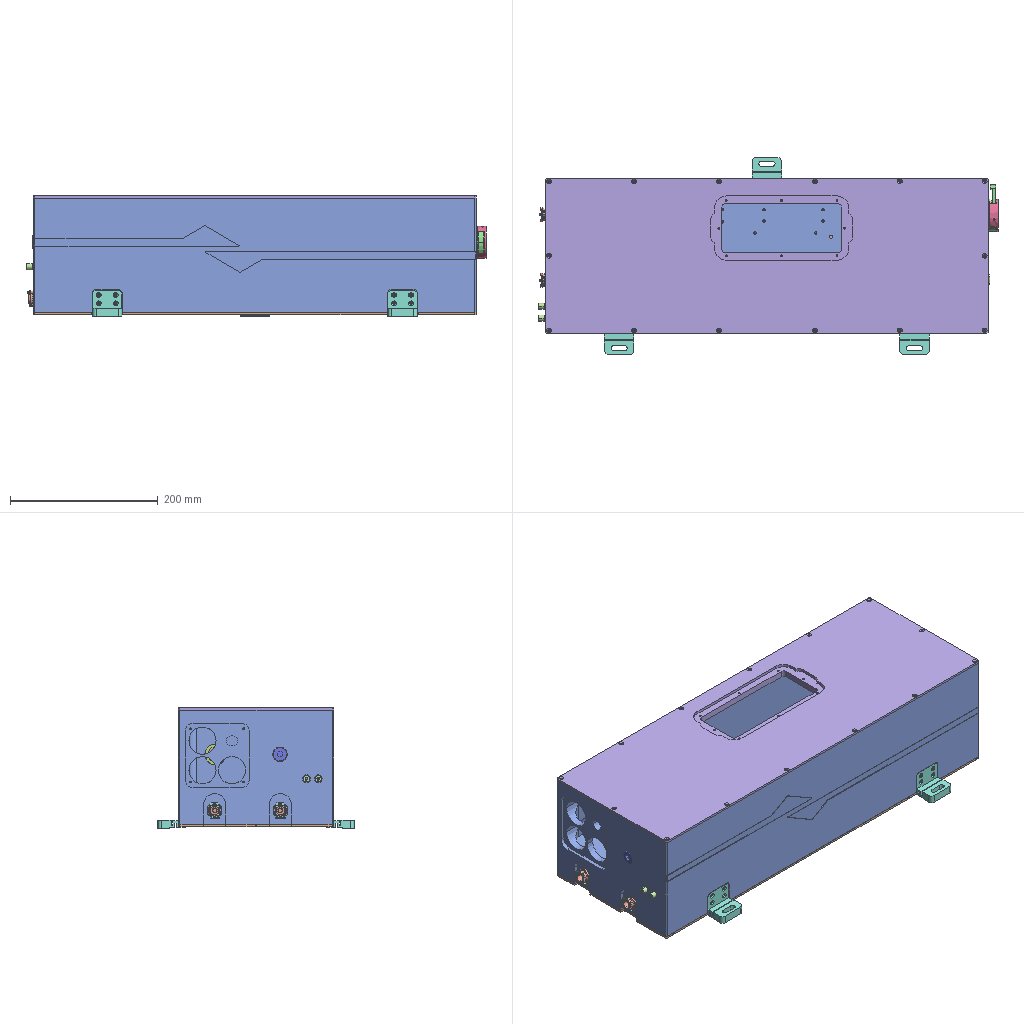Assembly | SolidWorks | 17 different items | 25 placed | box 623 x 266 x 163 mm
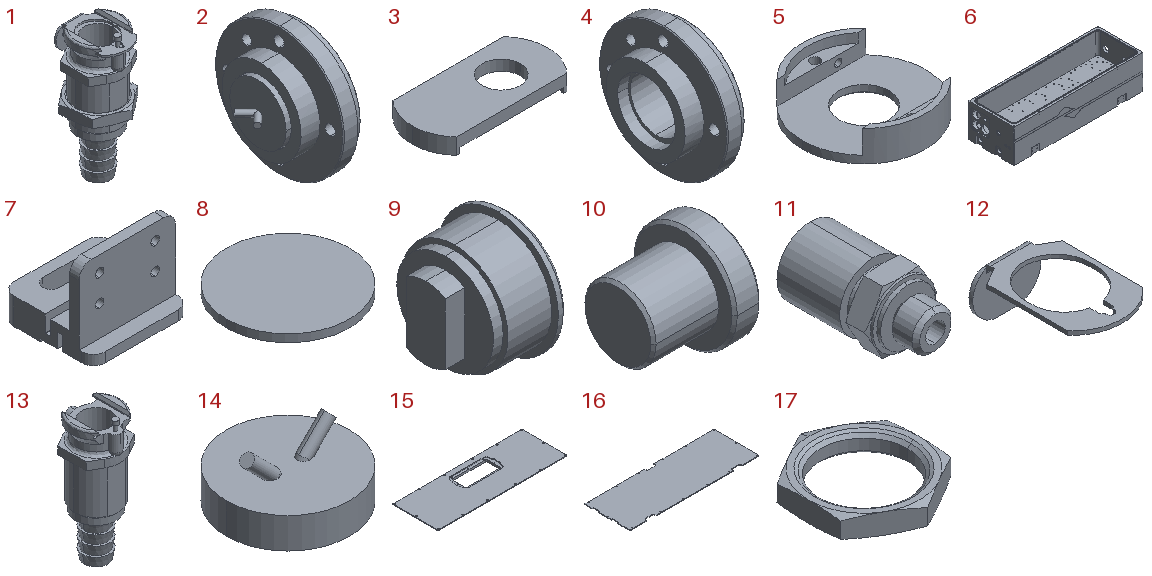Parts list (item | name | quantity | parent item | size | volume | features):
1 | (subassembly) | x2 | - | 22.024 x 23.624 x 51.054 mm | 6283 mm3 | -
2 | (subassembly) | x1 | - | 20.175 x 44 x 44 mm | 12487 mm3 | -
3 | - | x1 | - | 64 x 30 x 7.5 mm | 7628 mm3 | features ICE 5, 3DProfileFeature 2, HoleWzd 2, Extrusion 1
4 | - | x1 | in 2 | 14.489 x 44 x 44 mm | 10850 mm3 | features ICE 5, Chamfer 2, Revolution 1
5 | - | x1 | - | 44 x 44 x 11 mm | 5108 mm3 | features ICE 7, Chamfer 2, CirPattern 1, Extrusion 1
6 | - | x1 | - | 600 x 210 x 155 mm | 5602936 mm3 | features ICE 64, Fillet 20, 3DProfileFeature 18, HoleWzd 18, MoveFace 7, Chamfer 2, CirPattern 2, Cut 2, Extrusion 1, LPattern 1, MirrorPattern 1
7 | - | x3 | - | 40 x 38 x 35 mm | 14882 mm3 | features ICE 7, Fillet 3, MoveFace 3, Chamfer 1, Extrusion 1
8 | - | x1 | - | 16 x 16 x 1 mm | 201.062 mm3 | features Extrusion 1
9 | - | x1 | - | 19 x 24.8 x 24.8 mm | 5733 mm3 | features ICE 2, Revolution 2, Chamfer 1
10 | - | x1 | - | 17 x 19 x 19 mm | 2888 mm3 | features Chamfer 1, ICE 1, Revolution 1
11 | - | x3 | - | 9.238 x 16.5 x 8.5 mm | 660.447 mm3 | features BaseBody 1
12 | - | x2 | in 1 | 14.097 x 22.301 x 9.652 mm | 165.496 mm3 | features BaseBody 1
13 | - | x2 | in 1 | 19.05 x 19.99 x 51.054 mm | 5563 mm3 | features BaseBody 1
14 | - | x1 | in 2 | 20 x 20 x 14.516 mm | 1637 mm3 | features Sweep 2, Extrusion 1, MirrorPattern 1
15 | - | x1 | - | 600 x 210 x 13 mm | 425401 mm3 | features ICE 7, Fillet 4, Chamfer 2, 3DProfileFeature 1, Extrusion 1, HoleWzd 1
16 | - | x1 | - | 600 x 210 x 3 mm | 372208 mm3 | features Chamfer 2, ICE 2, Cut 1, Extrusion 1, Fillet 1, MoveFace 1
17 | - | x2 | in 1 | 20.638 x 23.83 x 3.81 mm | 553.998 mm3 | features BaseBody 1
Mates (type | each side: item.copy, entity, surface, feature):
In the top assembly
Coincident | assembly face | 6.1 face
Width | 6.1 face | 6.1 face | assembly face | assembly face
Coincident | assembly face | assembly face | 21 times
Concentric | assembly face | assembly face | 26 times
Coincident | 6.1 face plane Boss-Extrude1 | assembly face | 5 times
Coincident | 6.1 face plane Cut-Extrude1 | assembly face | 29 times
Parallel | 6.1 face plane Cut-Extrude1 | assembly face | 17 times
Concentric | assembly axis | assembly select_type:0 | 2 times
Coincident | assembly axis | assembly axis
Concentric | assembly axis | assembly face
DistanceDim | assembly face | assembly face | 12 times
Coincident | assembly select_type:0 | assembly select_type:0
Concentric | 6.1 face | assembly face | 11 times
DistanceDim | 6.1 face plane Cut-Extrude1 | assembly edge
DistanceDim | assembly face | 6.1 face plane Cut-Extrude1 | 10 times
DistanceDim | 6.1 face plane Cut-Extrude1 | assembly face | 5 times
Coincident | 6.1 face | assembly face | 9 times
Concentric | 6.1 face cylinder Cut-Extrude16 | assembly face
Coincident | 6.1 face plane Cut-Extrude15 | assembly face
Concentric | 6.1 face cylinder Cut-Extrude16 | 4.1 face cylinder Revolve1
Coincident | 6.1 face plane Cut-Extrude15 | 4.1 face plane Revolve1
Parallel | 6.1 face | assembly face | 3 times
DistanceDim | assembly select_type:0 | 6.1 face plane Cut-Extrude1
DistanceDim | assembly face | 6.1 face plane Boss-Extrude1 | 2 times
Coincident | 6.1 face plane Cut-Extrude19 | 7.1 face plane Boss-Extrude2
Coincident | 6.1 face plane Boss-Extrude1 | 7.1 face plane Boss-Extrude1
Width | 7.1 face plane Boss-Extrude1 | 7.1 face plane Boss-Extrude1 | 6.1 face plane Cut-Extrude19 | 6.1 face plane Cut-Extrude19
Coincident | 6.1 face plane Boss-Extrude1 | 7.2 face plane Boss-Extrude1
Coincident | 6.1 face plane Cut-Extrude19 | 7.2 face plane Boss-Extrude2
Width | 7.2 face plane Boss-Extrude1 | 7.2 face plane Boss-Extrude1 | 6.1 face plane Cut-Extrude19 | 6.1 face plane Cut-Extrude19
Coincident | 6.1 face plane Boss-Extrude1 | 7.3 face plane Boss-Extrude1
Coincident | 6.1 face plane Cut-Extrude18 | 7.3 face plane Boss-Extrude2
Width | 6.1 face plane Cut-Extrude18 | 6.1 face plane Cut-Extrude18 | 7.3 face plane Boss-Extrude1 | 7.3 face plane Boss-Extrude1
Coincident | 6.1 face plane Boss-Extrude1 | 16.1 face plane Boss-Extrude1 | 3 times
Coincident | 6.1 face plane Boss-Extrude1 | 15.1 face plane Boss-Extrude1 | 3 times
Coincident | 15.1 face | assembly face
Width | 15.1 face | 15.1 face | assembly face | assembly face | 2 times
Concentric | 4.1 face cylinder Cut-Extrude3 | 6.1 face cylinder CirPattern4
Parallel | 16.1 face plane Boss-Extrude1 | assembly face
Width | assembly face | assembly face | assembly face | assembly face
Coincident | 4.1 face plane Boss-Extrude1 | 3.1 face plane Boss-Extrude1
Parallel | 6.1 face plane Boss-Extrude1 | 3.1 face plane Boss-Extrude1
Coincident | 4.1 face plane Revolve1 | 5.1 face plane Boss-Extrude1
Concentric | 4.1 face cylinder Revolve1 | 5.1 face cylinder Boss-Extrude1
Concentric | 4.1 face cylinder Cut-Extrude3 | 5.1 face cylinder Cut-Extrude3
Concentric | 4.1 face cylinder Revolve1 | 3.1 face cylinder Boss-Extrude1
Concentric | 3.1 face cylinder Cut-Extrude1 | 8.1 face cylinder Boss-Extrude1
Coincident | 3.1 face plane Cut-Extrude1 | 8.1 face plane Boss-Extrude1
Coincident | 6.1 face plane Cut-Extrude2 | assembly face | 7 times
Parallel | 6.1 face plane Cut-Extrude2 | assembly face | 2 times
Coincident | 6.1 face plane Cut-Extrude38 | assembly face
Concentric | 6.1 face cylinder Cut-Extrude38 | assembly face
Concentric | 6.1 face cylinder Cut-Extrude41 | 9.1 face cylinder Revolve1
Coincident | 6.1 face plane Cut-Extrude42 | 9.1 face plane Revolve1
InPlace | 6.1 face plane Cut-Extrude46 | assembly plane
InPlace | 6.1 face | assembly plane
DistanceDim | 6.1 face plane Cut-Extrude2 | assembly face
Parallel | 6.1 face plane Boss-Extrude1 | assembly face
Concentric | 6.1 face cylinder Cut-Extrude53 | assembly face | 2 times
Concentric | 6.1 face cylinder Cut-Extrude38 | 10.1 face cylinder Revolve1
Coincident | 6.1 face plane Cut-Extrude38 | 10.1 face plane Revolve1
Concentric | 6.1 face cylinder Cut-Extrude55 | 11.1 face cylinder MS_5H_6
Coincident | 6.1 face plane Cut-Extrude56 | 11.1 face plane MS_5H_6
Coincident | 6.1 face plane Cut-Extrude56 | 11.2 face plane MS_5H_6
Concentric | 6.1 face cylinder Cut-Extrude55 | 11.2 face cylinder MS_5H_6
Coincident | 6.1 face plane Cut-Extrude1 | 11.3 face plane MS_5H_6
Concentric | 6.1 face cylinder Cut-Extrude55 | 11.3 face cylinder MS_5H_6
Concentric | 6.1 face cylinder Cut-Extrude55 | assembly face
Concentric | assembly face | assembly select_type:0
Coincident | 6.1 face plane Cut-Extrude3 | 13.1 face plane Input1
Coincident | 6.1 face plane Cut-Extrude3 | 13.2 face plane Input1
Parallel | 6.1 face plane Boss-Extrude23 | 13.2 face plane Input1
Concentric | 6.1 face cylinder Cut-Extrude66 | 13.1 face cylinder Input1
Concentric | 6.1 face cylinder Cut-Extrude66 | 13.2 face cylinder Input1
Concentric | 6.1 face cylinder Cut-Extrude67 | assembly face
Concentric | 7.1 face cylinder Cut-Extrude4 | assembly face | 2 times
Coincident | 7.1 face plane Boss-Extrude2 | assembly face
In subassembly 2
Coincident | 4.2 face plane Cut-Extrude2 | 14.1 face plane Boss-Extrude1
Concentric | 4.2 face cylinder Cut-Extrude2 | 14.1 face cylinder Boss-Extrude1
Concentric | 4.2 face cylinder Cut-Extrude2 | 2.1 face
Coincident | 4.2 plane | 14.1 plane
In subassembly 1
Concentric | 17.1 face cylinder Input1 | 13.3 face cylinder Input1
DistanceDim | 13.3 face plane Input1 | 17.1 face plane Input1